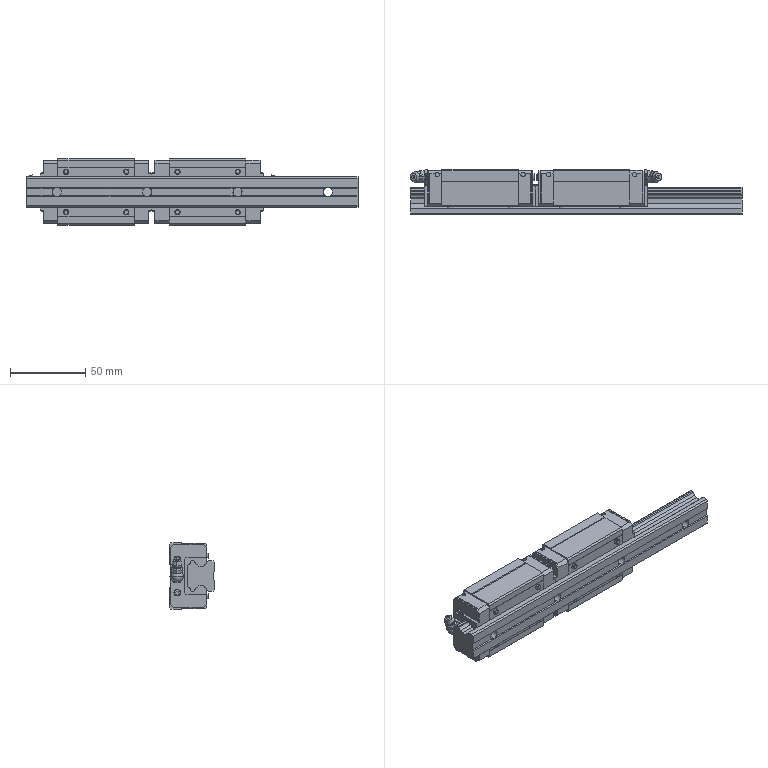Part | SolidWorks | 5 solids | 650 faces | box 220.441 x 30 x 44 mm | volume 182432 mm3 | plane 374 | cylinder 148 | cone 72 | torus 44 | sphere 12 | commonest cylinder face diameters 4.134 x32 6 x20 3 x16 3.43 x16 4.5 x16 4.917 x16